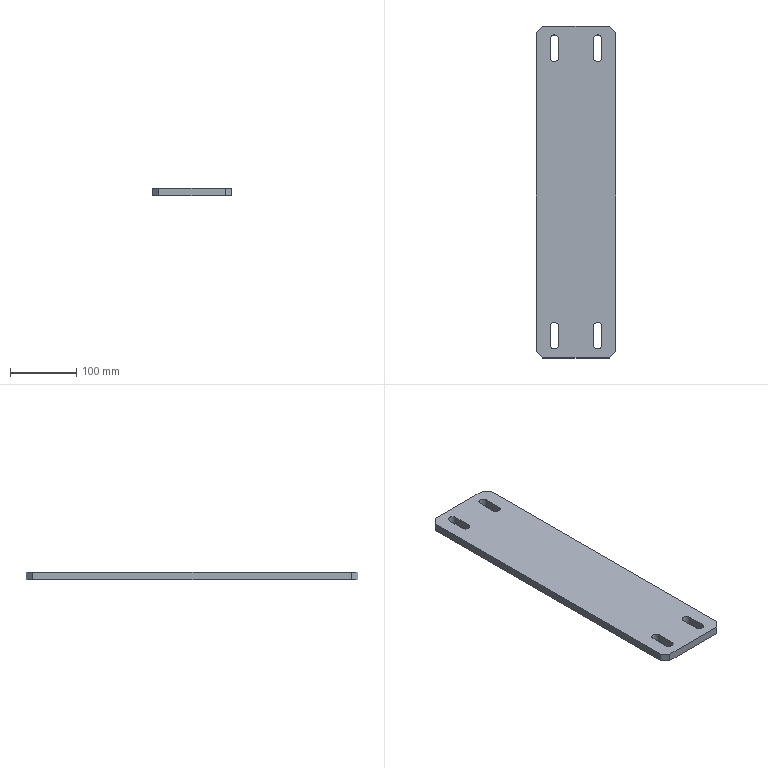Part | SolidWorks | features Chamfer 1, Extrusion 1, ICE 1 | 1 solid | 26 faces | box 120 x 500 x 12 mm | volume 694381 mm3 | plane 18 | cylinder 8 | commonest cylinder face diameters 13 x8
STEP:
#1=CARTESIAN_POINT('',(60.,-240.,12.));
#2=VERTEX_POINT('',#1);
#3=CARTESIAN_POINT('',(60.,240.,12.));
#4=VERTEX_POINT('',#3);
#5=CARTESIAN_POINT('',(60.,250.,12.));
#6=DIRECTION('',(0.,1.,0.));
#7=VECTOR('',#6,1000.);
#8=LINE('',#5,#7);
#9=EDGE_CURVE('',#2,#4,#8,.T.);
#10=ORIENTED_EDGE('',*,*,#9,.F.);
#11=CARTESIAN_POINT('',(60.,-240.,0.));
#12=VERTEX_POINT('',#11);
#13=CARTESIAN_POINT('',(60.,-240.,12.));
#14=DIRECTION('',(0.,0.,-1.));
#15=VECTOR('',#14,1000.);
#16=LINE('',#13,#15);
#17=EDGE_CURVE('',#2,#12,#16,.T.);
#18=ORIENTED_EDGE('',*,*,#17,.T.);
#19=CARTESIAN_POINT('',(60.,240.,0.));
#20=VERTEX_POINT('',#19);
#21=CARTESIAN_POINT('',(60.,250.,0.));
#22=DIRECTION('',(0.,1.,0.));
#23=VECTOR('',#22,1000.);
#24=LINE('',#21,#23);
#25=EDGE_CURVE('',#12,#20,#24,.T.);
#26=ORIENTED_EDGE('',*,*,#25,.T.);
#27=CARTESIAN_POINT('',(60.,240.,12.));
#28=DIRECTION('',(0.,0.,1.));
#29=VECTOR('',#28,1000.);
#30=LINE('',#27,#29);
#31=EDGE_CURVE('',#20,#4,#30,.T.);
#32=ORIENTED_EDGE('',*,*,#31,.T.);
#33=EDGE_LOOP('',(#10,#18,#26,#32));
#34=FACE_OUTER_BOUND('',#33,.T.);
#35=CARTESIAN_POINT('',(60.,250.,12.));
#36=DIRECTION('',(-1.,0.,0.));
#37=DIRECTION('',(0.,-1.,0.));
#38=AXIS2_PLACEMENT_3D('',#35,#36,#37);
#39=PLANE('',#38);
#40=ADVANCED_FACE('',(#34),#39,.F.);
#41=CARTESIAN_POINT('',(50.,250.,12.));
#42=VERTEX_POINT('',#41);
#43=CARTESIAN_POINT('',(-50.,250.,12.));
#44=VERTEX_POINT('',#43);
#45=CARTESIAN_POINT('',(-60.,250.,12.));
#46=DIRECTION('',(-1.,0.,0.));
#47=VECTOR('',#46,1000.);
#48=LINE('',#45,#47);
#49=EDGE_CURVE('',#42,#44,#48,.T.);
#50=ORIENTED_EDGE('',*,*,#49,.F.);
#51=CARTESIAN_POINT('',(50.,250.,0.));
#52=VERTEX_POINT('',#51);
#53=CARTESIAN_POINT('',(50.,250.,12.));
#54=DIRECTION('',(0.,0.,-1.));
#55=VECTOR('',#54,1000.);
#56=LINE('',#53,#55);
#57=EDGE_CURVE('',#42,#52,#56,.T.);
#58=ORIENTED_EDGE('',*,*,#57,.T.);
#59=CARTESIAN_POINT('',(-50.,250.,0.));
#60=VERTEX_POINT('',#59);
#61=CARTESIAN_POINT('',(-60.,250.,0.));
#62=DIRECTION('',(-1.,0.,0.));
#63=VECTOR('',#62,1000.);
#64=LINE('',#61,#63);
#65=EDGE_CURVE('',#52,#60,#64,.T.);
#66=ORIENTED_EDGE('',*,*,#65,.T.);
#67=CARTESIAN_POINT('',(-50.,250.,12.));
#68=DIRECTION('',(0.,0.,1.));
#69=VECTOR('',#68,1000.);
#70=LINE('',#67,#69);
#71=EDGE_CURVE('',#60,#44,#70,.T.);
#72=ORIENTED_EDGE('',*,*,#71,.T.);
#73=EDGE_LOOP('',(#50,#58,#66,#72));
#74=FACE_OUTER_BOUND('',#73,.T.);
#75=CARTESIAN_POINT('',(-60.,250.,12.));
#76=DIRECTION('',(0.,-1.,0.));
#77=DIRECTION('',(0.,0.,-1.));
#78=AXIS2_PLACEMENT_3D('',#75,#76,#77);
#79=PLANE('',#78);
#80=ADVANCED_FACE('',(#74),#79,.F.);
#81=CARTESIAN_POINT('',(-60.,240.,0.));
#82=VERTEX_POINT('',#81);
#83=CARTESIAN_POINT('',(-60.,-240.,0.));
#84=VERTEX_POINT('',#83);
#85=CARTESIAN_POINT('',(-60.,250.,0.));
#86=DIRECTION('',(0.,-1.,0.));
#87=VECTOR('',#86,1000.);
#88=LINE('',#85,#87);
#89=EDGE_CURVE('',#82,#84,#88,.T.);
#90=ORIENTED_EDGE('',*,*,#89,.T.);
#91=CARTESIAN_POINT('',(-60.,-240.,12.));
#92=VERTEX_POINT('',#91);
#93=CARTESIAN_POINT('',(-60.,-240.,12.));
#94=DIRECTION('',(0.,0.,1.));
#95=VECTOR('',#94,1000.);
#96=LINE('',#93,#95);
#97=EDGE_CURVE('',#84,#92,#96,.T.);
#98=ORIENTED_EDGE('',*,*,#97,.T.);
#99=CARTESIAN_POINT('',(-60.,240.,12.));
#100=VERTEX_POINT('',#99);
#101=CARTESIAN_POINT('',(-60.,250.,12.));
#102=DIRECTION('',(0.,-1.,0.));
#103=VECTOR('',#102,1000.);
#104=LINE('',#101,#103);
#105=EDGE_CURVE('',#100,#92,#104,.T.);
#106=ORIENTED_EDGE('',*,*,#105,.F.);
#107=CARTESIAN_POINT('',(-60.,240.,12.));
#108=DIRECTION('',(0.,0.,-1.));
#109=VECTOR('',#108,1000.);
#110=LINE('',#107,#109);
#111=EDGE_CURVE('',#100,#82,#110,.T.);
#112=ORIENTED_EDGE('',*,*,#111,.T.);
#113=EDGE_LOOP('',(#90,#98,#106,#112));
#114=FACE_OUTER_BOUND('',#113,.T.);
#115=CARTESIAN_POINT('',(-60.,250.,12.));
#116=DIRECTION('',(1.,0.,0.));
#117=DIRECTION('',(0.,1.,0.));
#118=AXIS2_PLACEMENT_3D('',#115,#116,#117);
#119=PLANE('',#118);
#120=ADVANCED_FACE('',(#114),#119,.F.);
#121=CARTESIAN_POINT('',(-50.,-250.,0.));
#122=VERTEX_POINT('',#121);
#123=CARTESIAN_POINT('',(50.,-250.,0.));
#124=VERTEX_POINT('',#123);
#125=CARTESIAN_POINT('',(-60.,-250.,0.));
#126=DIRECTION('',(1.,0.,0.));
#127=VECTOR('',#126,1000.);
#128=LINE('',#125,#127);
#129=EDGE_CURVE('',#122,#124,#128,.T.);
#130=ORIENTED_EDGE('',*,*,#129,.T.);
#131=CARTESIAN_POINT('',(50.,-250.,12.));
#132=VERTEX_POINT('',#131);
#133=CARTESIAN_POINT('',(50.,-250.,12.));
#134=DIRECTION('',(0.,0.,1.));
#135=VECTOR('',#134,1000.);
#136=LINE('',#133,#135);
#137=EDGE_CURVE('',#124,#132,#136,.T.);
#138=ORIENTED_EDGE('',*,*,#137,.T.);
#139=CARTESIAN_POINT('',(-50.,-250.,12.));
#140=VERTEX_POINT('',#139);
#141=CARTESIAN_POINT('',(-60.,-250.,12.));
#142=DIRECTION('',(1.,0.,0.));
#143=VECTOR('',#142,1000.);
#144=LINE('',#141,#143);
#145=EDGE_CURVE('',#140,#132,#144,.T.);
#146=ORIENTED_EDGE('',*,*,#145,.F.);
#147=CARTESIAN_POINT('',(-50.,-250.,12.));
#148=DIRECTION('',(0.,0.,-1.));
#149=VECTOR('',#148,1000.);
#150=LINE('',#147,#149);
#151=EDGE_CURVE('',#140,#122,#150,.T.);
#152=ORIENTED_EDGE('',*,*,#151,.T.);
#153=EDGE_LOOP('',(#130,#138,#146,#152));
#154=FACE_OUTER_BOUND('',#153,.T.);
#155=CARTESIAN_POINT('',(-60.,-250.,12.));
#156=DIRECTION('',(0.,1.,0.));
#157=DIRECTION('',(0.,0.,1.));
#158=AXIS2_PLACEMENT_3D('',#155,#156,#157);
#159=PLANE('',#158);
#160=ADVANCED_FACE('',(#154),#159,.F.);
#161=CARTESIAN_POINT('',(-39.,-230.,12.));
#162=VERTEX_POINT('',#161);
#163=CARTESIAN_POINT('',(-26.,-230.,12.));
#164=VERTEX_POINT('',#163);
#165=CARTESIAN_POINT('',(-32.5,-230.,12.));
#166=DIRECTION('',(0.,0.,1.));
#167=DIRECTION('',(-1.,0.,0.));
#168=AXIS2_PLACEMENT_3D('',#165,#166,#167);
#169=CIRCLE('',#168,6.5);
#170=EDGE_CURVE('',#162,#164,#169,.T.);
#171=ORIENTED_EDGE('',*,*,#170,.F.);
#172=CARTESIAN_POINT('',(-39.,-203.,12.));
#173=VERTEX_POINT('',#172);
#174=CARTESIAN_POINT('',(-39.,-230.,12.));
#175=DIRECTION('',(0.,-1.,0.));
#176=VECTOR('',#175,1000.);
#177=LINE('',#174,#176);
#178=EDGE_CURVE('',#173,#162,#177,.T.);
#179=ORIENTED_EDGE('',*,*,#178,.F.);
#180=CARTESIAN_POINT('',(-26.,-203.,12.));
#181=VERTEX_POINT('',#180);
#182=CARTESIAN_POINT('',(-32.5,-203.,12.));
#183=DIRECTION('',(0.,0.,1.));
#184=DIRECTION('',(-1.,0.,0.));
#185=AXIS2_PLACEMENT_3D('',#182,#183,#184);
#186=CIRCLE('',#185,6.5);
#187=EDGE_CURVE('',#181,#173,#186,.T.);
#188=ORIENTED_EDGE('',*,*,#187,.F.);
#189=CARTESIAN_POINT('',(-26.,-230.,12.));
#190=DIRECTION('',(0.,1.,0.));
#191=VECTOR('',#190,1000.);
#192=LINE('',#189,#191);
#193=EDGE_CURVE('',#164,#181,#192,.T.);
#194=ORIENTED_EDGE('',*,*,#193,.F.);
#195=EDGE_LOOP('',(#171,#179,#188,#194));
#196=FACE_BOUND('',#195,.T.);
#197=CARTESIAN_POINT('',(26.,-230.,12.));
#198=VERTEX_POINT('',#197);
#199=CARTESIAN_POINT('',(39.,-230.,12.));
#200=VERTEX_POINT('',#199);
#201=CARTESIAN_POINT('',(32.5,-230.,12.));
#202=DIRECTION('',(0.,0.,1.));
#203=DIRECTION('',(1.,0.,0.));
#204=AXIS2_PLACEMENT_3D('',#201,#202,#203);
#205=CIRCLE('',#204,6.5);
#206=EDGE_CURVE('',#198,#200,#205,.T.);
#207=ORIENTED_EDGE('',*,*,#206,.F.);
#208=CARTESIAN_POINT('',(26.,-203.,12.));
#209=VERTEX_POINT('',#208);
#210=CARTESIAN_POINT('',(26.,-230.,12.));
#211=DIRECTION('',(0.,-1.,0.));
#212=VECTOR('',#211,1000.);
#213=LINE('',#210,#212);
#214=EDGE_CURVE('',#209,#198,#213,.T.);
#215=ORIENTED_EDGE('',*,*,#214,.F.);
#216=CARTESIAN_POINT('',(39.,-203.,12.));
#217=VERTEX_POINT('',#216);
#218=CARTESIAN_POINT('',(32.5,-203.,12.));
#219=DIRECTION('',(0.,0.,1.));
#220=DIRECTION('',(1.,0.,0.));
#221=AXIS2_PLACEMENT_3D('',#218,#219,#220);
#222=CIRCLE('',#221,6.5);
#223=EDGE_CURVE('',#217,#209,#222,.T.);
#224=ORIENTED_EDGE('',*,*,#223,.F.);
#225=CARTESIAN_POINT('',(39.,-230.,12.));
#226=DIRECTION('',(0.,1.,0.));
#227=VECTOR('',#226,1000.);
#228=LINE('',#225,#227);
#229=EDGE_CURVE('',#200,#217,#228,.T.);
#230=ORIENTED_EDGE('',*,*,#229,.F.);
#231=EDGE_LOOP('',(#207,#215,#224,#230));
#232=FACE_BOUND('',#231,.T.);
#233=CARTESIAN_POINT('',(39.,230.,12.));
#234=VERTEX_POINT('',#233);
#235=CARTESIAN_POINT('',(26.,230.,12.));
#236=VERTEX_POINT('',#235);
#237=CARTESIAN_POINT('',(32.5,230.,12.));
#238=DIRECTION('',(0.,0.,1.));
#239=DIRECTION('',(-1.,0.,0.));
#240=AXIS2_PLACEMENT_3D('',#237,#238,#239);
#241=CIRCLE('',#240,6.5);
#242=EDGE_CURVE('',#234,#236,#241,.T.);
#243=ORIENTED_EDGE('',*,*,#242,.F.);
#244=CARTESIAN_POINT('',(39.,203.,12.));
#245=VERTEX_POINT('',#244);
#246=CARTESIAN_POINT('',(39.,230.,12.));
#247=DIRECTION('',(0.,1.,0.));
#248=VECTOR('',#247,1000.);
#249=LINE('',#246,#248);
#250=EDGE_CURVE('',#245,#234,#249,.T.);
#251=ORIENTED_EDGE('',*,*,#250,.F.);
#252=CARTESIAN_POINT('',(26.,203.,12.));
#253=VERTEX_POINT('',#252);
#254=CARTESIAN_POINT('',(32.5,203.,12.));
#255=DIRECTION('',(0.,0.,1.));
#256=DIRECTION('',(-1.,0.,0.));
#257=AXIS2_PLACEMENT_3D('',#254,#255,#256);
#258=CIRCLE('',#257,6.5);
#259=EDGE_CURVE('',#253,#245,#258,.T.);
#260=ORIENTED_EDGE('',*,*,#259,.F.);
#261=CARTESIAN_POINT('',(26.,230.,12.));
#262=DIRECTION('',(0.,-1.,0.));
#263=VECTOR('',#262,1000.);
#264=LINE('',#261,#263);
#265=EDGE_CURVE('',#236,#253,#264,.T.);
#266=ORIENTED_EDGE('',*,*,#265,.F.);
#267=EDGE_LOOP('',(#243,#251,#260,#266));
#268=FACE_BOUND('',#267,.T.);
#269=CARTESIAN_POINT('',(-26.,230.,12.));
#270=VERTEX_POINT('',#269);
#271=CARTESIAN_POINT('',(-39.,230.,12.));
#272=VERTEX_POINT('',#271);
#273=CARTESIAN_POINT('',(-32.5,230.,12.));
#274=DIRECTION('',(0.,0.,1.));
#275=DIRECTION('',(1.,0.,0.));
#276=AXIS2_PLACEMENT_3D('',#273,#274,#275);
#277=CIRCLE('',#276,6.5);
#278=EDGE_CURVE('',#270,#272,#277,.T.);
#279=ORIENTED_EDGE('',*,*,#278,.F.);
#280=CARTESIAN_POINT('',(-26.,203.,12.));
#281=VERTEX_POINT('',#280);
#282=CARTESIAN_POINT('',(-26.,230.,12.));
#283=DIRECTION('',(0.,1.,0.));
#284=VECTOR('',#283,1000.);
#285=LINE('',#282,#284);
#286=EDGE_CURVE('',#281,#270,#285,.T.);
#287=ORIENTED_EDGE('',*,*,#286,.F.);
#288=CARTESIAN_POINT('',(-39.,203.,12.));
#289=VERTEX_POINT('',#288);
#290=CARTESIAN_POINT('',(-32.5,203.,12.));
#291=DIRECTION('',(0.,0.,1.));
#292=DIRECTION('',(1.,0.,0.));
#293=AXIS2_PLACEMENT_3D('',#290,#291,#292);
#294=CIRCLE('',#293,6.5);
#295=EDGE_CURVE('',#289,#281,#294,.T.);
#296=ORIENTED_EDGE('',*,*,#295,.F.);
#297=CARTESIAN_POINT('',(-39.,230.,12.));
#298=DIRECTION('',(0.,-1.,0.));
#299=VECTOR('',#298,1000.);
#300=LINE('',#297,#299);
#301=EDGE_CURVE('',#272,#289,#300,.T.);
#302=ORIENTED_EDGE('',*,*,#301,.F.);
#303=EDGE_LOOP('',(#279,#287,#296,#302));
#304=FACE_BOUND('',#303,.T.);
#305=ORIENTED_EDGE('',*,*,#145,.T.);
#306=CARTESIAN_POINT('',(150.,-150.,12.));
#307=DIRECTION('',(0.7071,0.7071,0.));
#308=VECTOR('',#307,1000.);
#309=LINE('',#306,#308);
#310=EDGE_CURVE('',#132,#2,#309,.T.);
#311=ORIENTED_EDGE('',*,*,#310,.T.);
#312=ORIENTED_EDGE('',*,*,#9,.T.);
#313=CARTESIAN_POINT('',(150.,150.,12.));
#314=DIRECTION('',(-0.7071,0.7071,0.));
#315=VECTOR('',#314,1000.);
#316=LINE('',#313,#315);
#317=EDGE_CURVE('',#4,#42,#316,.T.);
#318=ORIENTED_EDGE('',*,*,#317,.T.);
#319=ORIENTED_EDGE('',*,*,#49,.T.);
#320=CARTESIAN_POINT('',(-150.,150.,12.));
#321=DIRECTION('',(-0.7071,-0.7071,0.));
#322=VECTOR('',#321,1000.);
#323=LINE('',#320,#322);
#324=EDGE_CURVE('',#44,#100,#323,.T.);
#325=ORIENTED_EDGE('',*,*,#324,.T.);
#326=ORIENTED_EDGE('',*,*,#105,.T.);
#327=CARTESIAN_POINT('',(-150.,-150.,12.));
#328=DIRECTION('',(0.7071,-0.7071,0.));
#329=VECTOR('',#328,1000.);
#330=LINE('',#327,#329);
#331=EDGE_CURVE('',#92,#140,#330,.T.);
#332=ORIENTED_EDGE('',*,*,#331,.T.);
#333=EDGE_LOOP('',(#305,#311,#312,#318,#319,#325,#326,#332));
#334=FACE_OUTER_BOUND('',#333,.T.);
#335=CARTESIAN_POINT('',(0.,0.,12.));
#336=DIRECTION('',(0.,0.,1.));
#337=DIRECTION('',(1.,0.,0.));
#338=AXIS2_PLACEMENT_3D('',#335,#336,#337);
#339=PLANE('',#338);
#340=ADVANCED_FACE('',(#196,#232,#268,#304,#334),#339,.T.);
#341=CARTESIAN_POINT('',(-39.,-203.,0.));
#342=VERTEX_POINT('',#341);
#343=CARTESIAN_POINT('',(-39.,-230.,0.));
#344=VERTEX_POINT('',#343);
#345=CARTESIAN_POINT('',(-39.,-230.,0.));
#346=DIRECTION('',(0.,-1.,0.));
#347=VECTOR('',#346,1000.);
#348=LINE('',#345,#347);
#349=EDGE_CURVE('',#342,#344,#348,.T.);
#350=ORIENTED_EDGE('',*,*,#349,.T.);
#351=CARTESIAN_POINT('',(-26.,-230.,0.));
#352=VERTEX_POINT('',#351);
#353=CARTESIAN_POINT('',(-32.5,-230.,0.));
#354=DIRECTION('',(0.,0.,1.));
#355=DIRECTION('',(-1.,0.,0.));
#356=AXIS2_PLACEMENT_3D('',#353,#354,#355);
#357=CIRCLE('',#356,6.5);
#358=EDGE_CURVE('',#344,#352,#357,.T.);
#359=ORIENTED_EDGE('',*,*,#358,.T.);
#360=CARTESIAN_POINT('',(-26.,-203.,0.));
#361=VERTEX_POINT('',#360);
#362=CARTESIAN_POINT('',(-26.,-230.,0.));
#363=DIRECTION('',(0.,1.,0.));
#364=VECTOR('',#363,1000.);
#365=LINE('',#362,#364);
#366=EDGE_CURVE('',#352,#361,#365,.T.);
#367=ORIENTED_EDGE('',*,*,#366,.T.);
#368=CARTESIAN_POINT('',(-32.5,-203.,0.));
#369=DIRECTION('',(0.,0.,1.));
#370=DIRECTION('',(-1.,0.,0.));
#371=AXIS2_PLACEMENT_3D('',#368,#369,#370);
#372=CIRCLE('',#371,6.5);
#373=EDGE_CURVE('',#361,#342,#372,.T.);
#374=ORIENTED_EDGE('',*,*,#373,.T.);
#375=EDGE_LOOP('',(#350,#359,#367,#374));
#376=FACE_BOUND('',#375,.T.);
#377=CARTESIAN_POINT('',(26.,-203.,0.));
#378=VERTEX_POINT('',#377);
#379=CARTESIAN_POINT('',(26.,-230.,0.));
#380=VERTEX_POINT('',#379);
#381=CARTESIAN_POINT('',(26.,-230.,0.));
#382=DIRECTION('',(0.,-1.,0.));
#383=VECTOR('',#382,1000.);
#384=LINE('',#381,#383);
#385=EDGE_CURVE('',#378,#380,#384,.T.);
#386=ORIENTED_EDGE('',*,*,#385,.T.);
#387=CARTESIAN_POINT('',(39.,-230.,0.));
#388=VERTEX_POINT('',#387);
#389=CARTESIAN_POINT('',(32.5,-230.,0.));
#390=DIRECTION('',(0.,0.,1.));
#391=DIRECTION('',(1.,0.,0.));
#392=AXIS2_PLACEMENT_3D('',#389,#390,#391);
#393=CIRCLE('',#392,6.5);
#394=EDGE_CURVE('',#380,#388,#393,.T.);
#395=ORIENTED_EDGE('',*,*,#394,.T.);
#396=CARTESIAN_POINT('',(39.,-203.,0.));
#397=VERTEX_POINT('',#396);
#398=CARTESIAN_POINT('',(39.,-230.,0.));
#399=DIRECTION('',(0.,1.,0.));
#400=VECTOR('',#399,1000.);
#401=LINE('',#398,#400);
#402=EDGE_CURVE('',#388,#397,#401,.T.);
#403=ORIENTED_EDGE('',*,*,#402,.T.);
#404=CARTESIAN_POINT('',(32.5,-203.,0.));
#405=DIRECTION('',(0.,0.,1.));
#406=DIRECTION('',(1.,0.,0.));
#407=AXIS2_PLACEMENT_3D('',#404,#405,#406);
#408=CIRCLE('',#407,6.5);
#409=EDGE_CURVE('',#397,#378,#408,.T.);
#410=ORIENTED_EDGE('',*,*,#409,.T.);
#411=EDGE_LOOP('',(#386,#395,#403,#410));
#412=FACE_BOUND('',#411,.T.);
#413=CARTESIAN_POINT('',(39.,203.,0.));
#414=VERTEX_POINT('',#413);
#415=CARTESIAN_POINT('',(39.,230.,0.));
#416=VERTEX_POINT('',#415);
#417=CARTESIAN_POINT('',(39.,230.,0.));
#418=DIRECTION('',(0.,1.,0.));
#419=VECTOR('',#418,1000.);
#420=LINE('',#417,#419);
#421=EDGE_CURVE('',#414,#416,#420,.T.);
#422=ORIENTED_EDGE('',*,*,#421,.T.);
#423=CARTESIAN_POINT('',(26.,230.,0.));
#424=VERTEX_POINT('',#423);
#425=CARTESIAN_POINT('',(32.5,230.,0.));
#426=DIRECTION('',(0.,0.,1.));
#427=DIRECTION('',(-1.,0.,0.));
#428=AXIS2_PLACEMENT_3D('',#425,#426,#427);
#429=CIRCLE('',#428,6.5);
#430=EDGE_CURVE('',#416,#424,#429,.T.);
#431=ORIENTED_EDGE('',*,*,#430,.T.);
#432=CARTESIAN_POINT('',(26.,203.,0.));
#433=VERTEX_POINT('',#432);
#434=CARTESIAN_POINT('',(26.,230.,0.));
#435=DIRECTION('',(0.,-1.,0.));
#436=VECTOR('',#435,1000.);
#437=LINE('',#434,#436);
#438=EDGE_CURVE('',#424,#433,#437,.T.);
#439=ORIENTED_EDGE('',*,*,#438,.T.);
#440=CARTESIAN_POINT('',(32.5,203.,0.));
#441=DIRECTION('',(0.,0.,1.));
#442=DIRECTION('',(-1.,0.,0.));
#443=AXIS2_PLACEMENT_3D('',#440,#441,#442);
#444=CIRCLE('',#443,6.5);
#445=EDGE_CURVE('',#433,#414,#444,.T.);
#446=ORIENTED_EDGE('',*,*,#445,.T.);
#447=EDGE_LOOP('',(#422,#431,#439,#446));
#448=FACE_BOUND('',#447,.T.);
#449=CARTESIAN_POINT('',(-26.,203.,0.));
#450=VERTEX_POINT('',#449);
#451=CARTESIAN_POINT('',(-26.,230.,0.));
#452=VERTEX_POINT('',#451);
#453=CARTESIAN_POINT('',(-26.,230.,0.));
#454=DIRECTION('',(0.,1.,0.));
#455=VECTOR('',#454,1000.);
#456=LINE('',#453,#455);
#457=EDGE_CURVE('',#450,#452,#456,.T.);
#458=ORIENTED_EDGE('',*,*,#457,.T.);
#459=CARTESIAN_POINT('',(-39.,230.,0.));
#460=VERTEX_POINT('',#459);
#461=CARTESIAN_POINT('',(-32.5,230.,0.));
#462=DIRECTION('',(0.,0.,1.));
#463=DIRECTION('',(1.,0.,0.));
#464=AXIS2_PLACEMENT_3D('',#461,#462,#463);
#465=CIRCLE('',#464,6.5);
#466=EDGE_CURVE('',#452,#460,#465,.T.);
#467=ORIENTED_EDGE('',*,*,#466,.T.);
#468=CARTESIAN_POINT('',(-39.,203.,0.));
#469=VERTEX_POINT('',#468);
#470=CARTESIAN_POINT('',(-39.,230.,0.));
#471=DIRECTION('',(0.,-1.,0.));
#472=VECTOR('',#471,1000.);
#473=LINE('',#470,#472);
#474=EDGE_CURVE('',#460,#469,#473,.T.);
#475=ORIENTED_EDGE('',*,*,#474,.T.);
#476=CARTESIAN_POINT('',(-32.5,203.,0.));
#477=DIRECTION('',(0.,0.,1.));
#478=DIRECTION('',(1.,0.,0.));
#479=AXIS2_PLACEMENT_3D('',#476,#477,#478);
#480=CIRCLE('',#479,6.5);
#481=EDGE_CURVE('',#469,#450,#480,.T.);
#482=ORIENTED_EDGE('',*,*,#481,.T.);
#483=EDGE_LOOP('',(#458,#467,#475,#482));
#484=FACE_BOUND('',#483,.T.);
#485=ORIENTED_EDGE('',*,*,#25,.F.);
#486=CARTESIAN_POINT('',(60.,-240.,0.));
#487=DIRECTION('',(-0.7071,-0.7071,0.));
#488=VECTOR('',#487,1000.);
#489=LINE('',#486,#488);
#490=EDGE_CURVE('',#12,#124,#489,.T.);
#491=ORIENTED_EDGE('',*,*,#490,.T.);
#492=ORIENTED_EDGE('',*,*,#129,.F.);
#493=CARTESIAN_POINT('',(-50.,-250.,0.));
#494=DIRECTION('',(-0.7071,0.7071,0.));
#495=VECTOR('',#494,1000.);
#496=LINE('',#493,#495);
#497=EDGE_CURVE('',#122,#84,#496,.T.);
#498=ORIENTED_EDGE('',*,*,#497,.T.);
#499=ORIENTED_EDGE('',*,*,#89,.F.);
#500=CARTESIAN_POINT('',(-60.,240.,0.));
#501=DIRECTION('',(0.7071,0.7071,0.));
#502=VECTOR('',#501,1000.);
#503=LINE('',#500,#502);
#504=EDGE_CURVE('',#82,#60,#503,.T.);
#505=ORIENTED_EDGE('',*,*,#504,.T.);
#506=ORIENTED_EDGE('',*,*,#65,.F.);
#507=CARTESIAN_POINT('',(50.,250.,0.));
#508=DIRECTION('',(0.7071,-0.7071,0.));
#509=VECTOR('',#508,1000.);
#510=LINE('',#507,#509);
#511=EDGE_CURVE('',#52,#20,#510,.T.);
#512=ORIENTED_EDGE('',*,*,#511,.T.);
#513=EDGE_LOOP('',(#485,#491,#492,#498,#499,#505,#506,#512));
#514=FACE_OUTER_BOUND('',#513,.T.);
#515=CARTESIAN_POINT('',(0.,0.,0.));
#516=DIRECTION('',(0.,0.,1.));
#517=DIRECTION('',(1.,0.,0.));
#518=AXIS2_PLACEMENT_3D('',#515,#516,#517);
#519=PLANE('',#518);
#520=ADVANCED_FACE('',(#376,#412,#448,#484,#514),#519,.F.);
#521=ORIENTED_EDGE('',*,*,#278,.T.);
#522=CARTESIAN_POINT('',(-39.,230.,0.));
#523=DIRECTION('',(0.,0.,1.));
#524=VECTOR('',#523,1000.);
#525=LINE('',#522,#524);
#526=EDGE_CURVE('',#460,#272,#525,.T.);
#527=ORIENTED_EDGE('',*,*,#526,.F.);
#528=ORIENTED_EDGE('',*,*,#466,.F.);
#529=CARTESIAN_POINT('',(-26.,230.,0.));
#530=DIRECTION('',(0.,0.,1.));
#531=VECTOR('',#530,1000.);
#532=LINE('',#529,#531);
#533=EDGE_CURVE('',#452,#270,#532,.T.);
#534=ORIENTED_EDGE('',*,*,#533,.T.);
#535=EDGE_LOOP('',(#521,#527,#528,#534));
#536=FACE_OUTER_BOUND('',#535,.T.);
#537=CARTESIAN_POINT('',(-32.5,230.,0.));
#538=DIRECTION('',(0.,0.,1.));
#539=DIRECTION('',(1.,0.,0.));
#540=AXIS2_PLACEMENT_3D('',#537,#538,#539);
#541=CYLINDRICAL_SURFACE('',#540,6.5);
#542=ADVANCED_FACE('',(#536),#541,.F.);
#543=ORIENTED_EDGE('',*,*,#286,.T.);
#544=ORIENTED_EDGE('',*,*,#533,.F.);
#545=ORIENTED_EDGE('',*,*,#457,.F.);
#546=CARTESIAN_POINT('',(-26.,203.,0.));
#547=DIRECTION('',(0.,0.,1.));
#548=VECTOR('',#547,1000.);
#549=LINE('',#546,#548);
#550=EDGE_CURVE('',#450,#281,#549,.T.);
#551=ORIENTED_EDGE('',*,*,#550,.T.);
#552=EDGE_LOOP('',(#543,#544,#545,#551));
#553=FACE_OUTER_BOUND('',#552,.T.);
#554=CARTESIAN_POINT('',(-26.,230.,0.));
#555=DIRECTION('',(1.,0.,0.));
#556=DIRECTION('',(0.,0.,-1.));
#557=AXIS2_PLACEMENT_3D('',#554,#555,#556);
#558=PLANE('',#557);
#559=ADVANCED_FACE('',(#553),#558,.F.);
#560=ORIENTED_EDGE('',*,*,#295,.T.);
#561=ORIENTED_EDGE('',*,*,#550,.F.);
#562=ORIENTED_EDGE('',*,*,#481,.F.);
#563=CARTESIAN_POINT('',(-39.,203.,0.));
#564=DIRECTION('',(0.,0.,1.));
#565=VECTOR('',#564,1000.);
#566=LINE('',#563,#565);
#567=EDGE_CURVE('',#469,#289,#566,.T.);
#568=ORIENTED_EDGE('',*,*,#567,.T.);
#569=EDGE_LOOP('',(#560,#561,#562,#568));
#570=FACE_OUTER_BOUND('',#569,.T.);
#571=CARTESIAN_POINT('',(-32.5,203.,0.));
#572=DIRECTION('',(0.,0.,1.));
#573=DIRECTION('',(1.,0.,0.));
#574=AXIS2_PLACEMENT_3D('',#571,#572,#573);
#575=CYLINDRICAL_SURFACE('',#574,6.5);
#576=ADVANCED_FACE('',(#570),#575,.F.);
#577=ORIENTED_EDGE('',*,*,#301,.T.);
#578=ORIENTED_EDGE('',*,*,#567,.F.);
#579=ORIENTED_EDGE('',*,*,#474,.F.);
#580=ORIENTED_EDGE('',*,*,#526,.T.);
#581=EDGE_LOOP('',(#577,#578,#579,#580));
#582=FACE_OUTER_BOUND('',#581,.T.);
#583=CARTESIAN_POINT('',(-39.,230.,0.));
#584=DIRECTION('',(-1.,0.,0.));
#585=DIRECTION('',(0.,-1.,0.));
#586=AXIS2_PLACEMENT_3D('',#583,#584,#585);
#587=PLANE('',#586);
#588=ADVANCED_FACE('',(#582),#587,.F.);
#589=ORIENTED_EDGE('',*,*,#242,.T.);
#590=CARTESIAN_POINT('',(26.,230.,0.));
#591=DIRECTION('',(0.,0.,1.));
#592=VECTOR('',#591,1000.);
#593=LINE('',#590,#592);
#594=EDGE_CURVE('',#424,#236,#593,.T.);
#595=ORIENTED_EDGE('',*,*,#594,.F.);
#596=ORIENTED_EDGE('',*,*,#430,.F.);
#597=CARTESIAN_POINT('',(39.,230.,0.));
#598=DIRECTION('',(0.,0.,1.));
#599=VECTOR('',#598,1000.);
#600=LINE('',#597,#599);
#601=EDGE_CURVE('',#416,#234,#600,.T.);
#602=ORIENTED_EDGE('',*,*,#601,.T.);
#603=EDGE_LOOP('',(#589,#595,#596,#602));
#604=FACE_OUTER_BOUND('',#603,.T.);
#605=CARTESIAN_POINT('',(32.5,230.,0.));
#606=DIRECTION('',(0.,0.,1.));
#607=DIRECTION('',(1.,0.,0.));
#608=AXIS2_PLACEMENT_3D('',#605,#606,#607);
#609=CYLINDRICAL_SURFACE('',#608,6.5);
#610=ADVANCED_FACE('',(#604),#609,.F.);
#611=ORIENTED_EDGE('',*,*,#250,.T.);
#612=ORIENTED_EDGE('',*,*,#601,.F.);
#613=ORIENTED_EDGE('',*,*,#421,.F.);
#614=CARTESIAN_POINT('',(39.,203.,0.));
#615=DIRECTION('',(0.,0.,1.));
#616=VECTOR('',#615,1000.);
#617=LINE('',#614,#616);
#618=EDGE_CURVE('',#414,#245,#617,.T.);
#619=ORIENTED_EDGE('',*,*,#618,.T.);
#620=EDGE_LOOP('',(#611,#612,#613,#619));
#621=FACE_OUTER_BOUND('',#620,.T.);
#622=CARTESIAN_POINT('',(39.,230.,0.));
#623=DIRECTION('',(1.,0.,0.));
#624=DIRECTION('',(0.,1.,0.));
#625=AXIS2_PLACEMENT_3D('',#622,#623,#624);
#626=PLANE('',#625);
#627=ADVANCED_FACE('',(#621),#626,.F.);
#628=ORIENTED_EDGE('',*,*,#259,.T.);
#629=ORIENTED_EDGE('',*,*,#618,.F.);
#630=ORIENTED_EDGE('',*,*,#445,.F.);
#631=CARTESIAN_POINT('',(26.,203.,0.));
#632=DIRECTION('',(0.,0.,1.));
#633=VECTOR('',#632,1000.);
#634=LINE('',#631,#633);
#635=EDGE_CURVE('',#433,#253,#634,.T.);
#636=ORIENTED_EDGE('',*,*,#635,.T.);
#637=EDGE_LOOP('',(#628,#629,#630,#636));
#638=FACE_OUTER_BOUND('',#637,.T.);
#639=CARTESIAN_POINT('',(32.5,203.,0.));
#640=DIRECTION('',(0.,0.,1.));
#641=DIRECTION('',(1.,0.,0.));
#642=AXIS2_PLACEMENT_3D('',#639,#640,#641);
#643=CYLINDRICAL_SURFACE('',#642,6.5);
#644=ADVANCED_FACE('',(#638),#643,.F.);
#645=ORIENTED_EDGE('',*,*,#265,.T.);
#646=ORIENTED_EDGE('',*,*,#635,.F.);
#647=ORIENTED_EDGE('',*,*,#438,.F.);
#648=ORIENTED_EDGE('',*,*,#594,.T.);
#649=EDGE_LOOP('',(#645,#646,#647,#648));
#650=FACE_OUTER_BOUND('',#649,.T.);
#651=CARTESIAN_POINT('',(26.,230.,0.));
#652=DIRECTION('',(-1.,0.,0.));
#653=DIRECTION('',(0.,-1.,0.));
#654=AXIS2_PLACEMENT_3D('',#651,#652,#653);
#655=PLANE('',#654);
#656=ADVANCED_FACE('',(#650),#655,.F.);
#657=ORIENTED_EDGE('',*,*,#206,.T.);
#658=CARTESIAN_POINT('',(39.,-230.,0.));
#659=DIRECTION('',(0.,0.,1.));
#660=VECTOR('',#659,1000.);
#661=LINE('',#658,#660);
#662=EDGE_CURVE('',#388,#200,#661,.T.);
#663=ORIENTED_EDGE('',*,*,#662,.F.);
#664=ORIENTED_EDGE('',*,*,#394,.F.);
#665=CARTESIAN_POINT('',(26.,-230.,0.));
#666=DIRECTION('',(0.,0.,1.));
#667=VECTOR('',#666,1000.);
#668=LINE('',#665,#667);
#669=EDGE_CURVE('',#380,#198,#668,.T.);
#670=ORIENTED_EDGE('',*,*,#669,.T.);
#671=EDGE_LOOP('',(#657,#663,#664,#670));
#672=FACE_OUTER_BOUND('',#671,.T.);
#673=CARTESIAN_POINT('',(32.5,-230.,0.));
#674=DIRECTION('',(0.,0.,1.));
#675=DIRECTION('',(1.,0.,0.));
#676=AXIS2_PLACEMENT_3D('',#673,#674,#675);
#677=CYLINDRICAL_SURFACE('',#676,6.5);
#678=ADVANCED_FACE('',(#672),#677,.F.);
#679=ORIENTED_EDGE('',*,*,#214,.T.);
#680=ORIENTED_EDGE('',*,*,#669,.F.);
#681=ORIENTED_EDGE('',*,*,#385,.F.);
#682=CARTESIAN_POINT('',(26.,-203.,0.));
#683=DIRECTION('',(0.,0.,1.));
#684=VECTOR('',#683,1000.);
#685=LINE('',#682,#684);
#686=EDGE_CURVE('',#378,#209,#685,.T.);
#687=ORIENTED_EDGE('',*,*,#686,.T.);
#688=EDGE_LOOP('',(#679,#680,#681,#687));
#689=FACE_OUTER_BOUND('',#688,.T.);
#690=CARTESIAN_POINT('',(26.,-230.,0.));
#691=DIRECTION('',(-1.,0.,0.));
#692=DIRECTION('',(0.,-1.,0.));
#693=AXIS2_PLACEMENT_3D('',#690,#691,#692);
#694=PLANE('',#693);
#695=ADVANCED_FACE('',(#689),#694,.F.);
#696=ORIENTED_EDGE('',*,*,#223,.T.);
#697=ORIENTED_EDGE('',*,*,#686,.F.);
#698=ORIENTED_EDGE('',*,*,#409,.F.);
#699=CARTESIAN_POINT('',(39.,-203.,0.));
#700=DIRECTION('',(0.,0.,1.));
#701=VECTOR('',#700,1000.);
#702=LINE('',#699,#701);
#703=EDGE_CURVE('',#397,#217,#702,.T.);
#704=ORIENTED_EDGE('',*,*,#703,.T.);
#705=EDGE_LOOP('',(#696,#697,#698,#704));
#706=FACE_OUTER_BOUND('',#705,.T.);
#707=CARTESIAN_POINT('',(32.5,-203.,0.));
#708=DIRECTION('',(0.,0.,1.));
#709=DIRECTION('',(1.,0.,0.));
#710=AXIS2_PLACEMENT_3D('',#707,#708,#709);
#711=CYLINDRICAL_SURFACE('',#710,6.5);
#712=ADVANCED_FACE('',(#706),#711,.F.);
#713=ORIENTED_EDGE('',*,*,#229,.T.);
#714=ORIENTED_EDGE('',*,*,#703,.F.);
#715=ORIENTED_EDGE('',*,*,#402,.F.);
#716=ORIENTED_EDGE('',*,*,#662,.T.);
#717=EDGE_LOOP('',(#713,#714,#715,#716));
#718=FACE_OUTER_BOUND('',#717,.T.);
#719=CARTESIAN_POINT('',(39.,-230.,0.));
#720=DIRECTION('',(1.,0.,0.));
#721=DIRECTION('',(0.,0.,-1.));
#722=AXIS2_PLACEMENT_3D('',#719,#720,#721);
#723=PLANE('',#722);
#724=ADVANCED_FACE('',(#718),#723,.F.);
#725=ORIENTED_EDGE('',*,*,#170,.T.);
#726=CARTESIAN_POINT('',(-26.,-230.,0.));
#727=DIRECTION('',(0.,0.,1.));
#728=VECTOR('',#727,1000.);
#729=LINE('',#726,#728);
#730=EDGE_CURVE('',#352,#164,#729,.T.);
#731=ORIENTED_EDGE('',*,*,#730,.F.);
#732=ORIENTED_EDGE('',*,*,#358,.F.);
#733=CARTESIAN_POINT('',(-39.,-230.,0.));
#734=DIRECTION('',(0.,0.,1.));
#735=VECTOR('',#734,1000.);
#736=LINE('',#733,#735);
#737=EDGE_CURVE('',#344,#162,#736,.T.);
#738=ORIENTED_EDGE('',*,*,#737,.T.);
#739=EDGE_LOOP('',(#725,#731,#732,#738));
#740=FACE_OUTER_BOUND('',#739,.T.);
#741=CARTESIAN_POINT('',(-32.5,-230.,0.));
#742=DIRECTION('',(0.,0.,1.));
#743=DIRECTION('',(1.,0.,0.));
#744=AXIS2_PLACEMENT_3D('',#741,#742,#743);
#745=CYLINDRICAL_SURFACE('',#744,6.5);
#746=ADVANCED_FACE('',(#740),#745,.F.);
#747=ORIENTED_EDGE('',*,*,#178,.T.);
#748=ORIENTED_EDGE('',*,*,#737,.F.);
#749=ORIENTED_EDGE('',*,*,#349,.F.);
#750=CARTESIAN_POINT('',(-39.,-203.,0.));
#751=DIRECTION('',(0.,0.,1.));
#752=VECTOR('',#751,1000.);
#753=LINE('',#750,#752);
#754=EDGE_CURVE('',#342,#173,#753,.T.);
#755=ORIENTED_EDGE('',*,*,#754,.T.);
#756=EDGE_LOOP('',(#747,#748,#749,#755));
#757=FACE_OUTER_BOUND('',#756,.T.);
#758=CARTESIAN_POINT('',(-39.,-230.,0.));
#759=DIRECTION('',(-1.,0.,0.));
#760=DIRECTION('',(0.,0.,1.));
#761=AXIS2_PLACEMENT_3D('',#758,#759,#760);
#762=PLANE('',#761);
#763=ADVANCED_FACE('',(#757),#762,.F.);
#764=ORIENTED_EDGE('',*,*,#187,.T.);
#765=ORIENTED_EDGE('',*,*,#754,.F.);
#766=ORIENTED_EDGE('',*,*,#373,.F.);
#767=CARTESIAN_POINT('',(-26.,-203.,0.));
#768=DIRECTION('',(0.,0.,1.));
#769=VECTOR('',#768,1000.);
#770=LINE('',#767,#769);
#771=EDGE_CURVE('',#361,#181,#770,.T.);
#772=ORIENTED_EDGE('',*,*,#771,.T.);
#773=EDGE_LOOP('',(#764,#765,#766,#772));
#774=FACE_OUTER_BOUND('',#773,.T.);
#775=CARTESIAN_POINT('',(-32.5,-203.,0.));
#776=DIRECTION('',(0.,0.,1.));
#777=DIRECTION('',(1.,0.,0.));
#778=AXIS2_PLACEMENT_3D('',#775,#776,#777);
#779=CYLINDRICAL_SURFACE('',#778,6.5);
#780=ADVANCED_FACE('',(#774),#779,.F.);
#781=ORIENTED_EDGE('',*,*,#193,.T.);
#782=ORIENTED_EDGE('',*,*,#771,.F.);
#783=ORIENTED_EDGE('',*,*,#366,.F.);
#784=ORIENTED_EDGE('',*,*,#730,.T.);
#785=EDGE_LOOP('',(#781,#782,#783,#784));
#786=FACE_OUTER_BOUND('',#785,.T.);
#787=CARTESIAN_POINT('',(-26.,-230.,0.));
#788=DIRECTION('',(1.,0.,0.));
#789=DIRECTION('',(0.,0.,-1.));
#790=AXIS2_PLACEMENT_3D('',#787,#788,#789);
#791=PLANE('',#790);
#792=ADVANCED_FACE('',(#786),#791,.F.);
#793=ORIENTED_EDGE('',*,*,#310,.F.);
#794=ORIENTED_EDGE('',*,*,#137,.F.);
#795=ORIENTED_EDGE('',*,*,#490,.F.);
#796=ORIENTED_EDGE('',*,*,#17,.F.);
#797=EDGE_LOOP('',(#793,#794,#795,#796));
#798=FACE_OUTER_BOUND('',#797,.T.);
#799=CARTESIAN_POINT('',(60.,-240.,12.));
#800=DIRECTION('',(-0.7071,0.7071,0.));
#801=DIRECTION('',(0.,0.,-1.));
#802=AXIS2_PLACEMENT_3D('',#799,#800,#801);
#803=PLANE('',#802);
#804=ADVANCED_FACE('',(#798),#803,.F.);
#805=ORIENTED_EDGE('',*,*,#331,.F.);
#806=ORIENTED_EDGE('',*,*,#97,.F.);
#807=ORIENTED_EDGE('',*,*,#497,.F.);
#808=ORIENTED_EDGE('',*,*,#151,.F.);
#809=EDGE_LOOP('',(#805,#806,#807,#808));
#810=FACE_OUTER_BOUND('',#809,.T.);
#811=CARTESIAN_POINT('',(-50.,-250.,12.));
#812=DIRECTION('',(0.7071,0.7071,0.));
#813=DIRECTION('',(0.,0.,-1.));
#814=AXIS2_PLACEMENT_3D('',#811,#812,#813);
#815=PLANE('',#814);
#816=ADVANCED_FACE('',(#810),#815,.F.);
#817=ORIENTED_EDGE('',*,*,#317,.F.);
#818=ORIENTED_EDGE('',*,*,#31,.F.);
#819=ORIENTED_EDGE('',*,*,#511,.F.);
#820=ORIENTED_EDGE('',*,*,#57,.F.);
#821=EDGE_LOOP('',(#817,#818,#819,#820));
#822=FACE_OUTER_BOUND('',#821,.T.);
#823=CARTESIAN_POINT('',(50.,250.,12.));
#824=DIRECTION('',(-0.7071,-0.7071,0.));
#825=DIRECTION('',(0.,0.,-1.));
#826=AXIS2_PLACEMENT_3D('',#823,#824,#825);
#827=PLANE('',#826);
#828=ADVANCED_FACE('',(#822),#827,.F.);
#829=ORIENTED_EDGE('',*,*,#324,.F.);
#830=ORIENTED_EDGE('',*,*,#71,.F.);
#831=ORIENTED_EDGE('',*,*,#504,.F.);
#832=ORIENTED_EDGE('',*,*,#111,.F.);
#833=EDGE_LOOP('',(#829,#830,#831,#832));
#834=FACE_OUTER_BOUND('',#833,.T.);
#835=CARTESIAN_POINT('',(-60.,240.,12.));
#836=DIRECTION('',(0.7071,-0.7071,0.));
#837=DIRECTION('',(0.,0.,-1.));
#838=AXIS2_PLACEMENT_3D('',#835,#836,#837);
#839=PLANE('',#838);
#840=ADVANCED_FACE('',(#834),#839,.F.);
#841=CLOSED_SHELL('',(#40,#80,#120,#160,#340,#520,#542,#559,#576,#588,#610,#627,#644,#656,#678,#695,#712,#724,#746,#763,#780,#792,#804,#816,#828,#840));
#842=MANIFOLD_SOLID_BREP('',#841);
#843=CARTESIAN_POINT('',(0.,0.,0.));
#844=DIRECTION('',(0.,0.,1.));
#845=DIRECTION('',(1.,0.,0.));
#846=AXIS2_PLACEMENT_3D('',#843,#844,#845);
#847=(LENGTH_UNIT()NAMED_UNIT(*)SI_UNIT(.MILLI.,.METRE.));
#848=UNCERTAINTY_MEASURE_WITH_UNIT(LENGTH_MEASURE(0.00001),#847,'','');
#849=(NAMED_UNIT(*)PLANE_ANGLE_UNIT()SI_UNIT($,.RADIAN.));
#850=(NAMED_UNIT(*)SI_UNIT($,.STERADIAN.)SOLID_ANGLE_UNIT());
#851=(GEOMETRIC_REPRESENTATION_CONTEXT(3)GLOBAL_UNCERTAINTY_ASSIGNED_CONTEXT((#848))GLOBAL_UNIT_ASSIGNED_CONTEXT((#847,#849,#850))REPRESENTATION_CONTEXT('',''));
#852=ADVANCED_BREP_SHAPE_REPRESENTATION('',(#842,#846),#851);